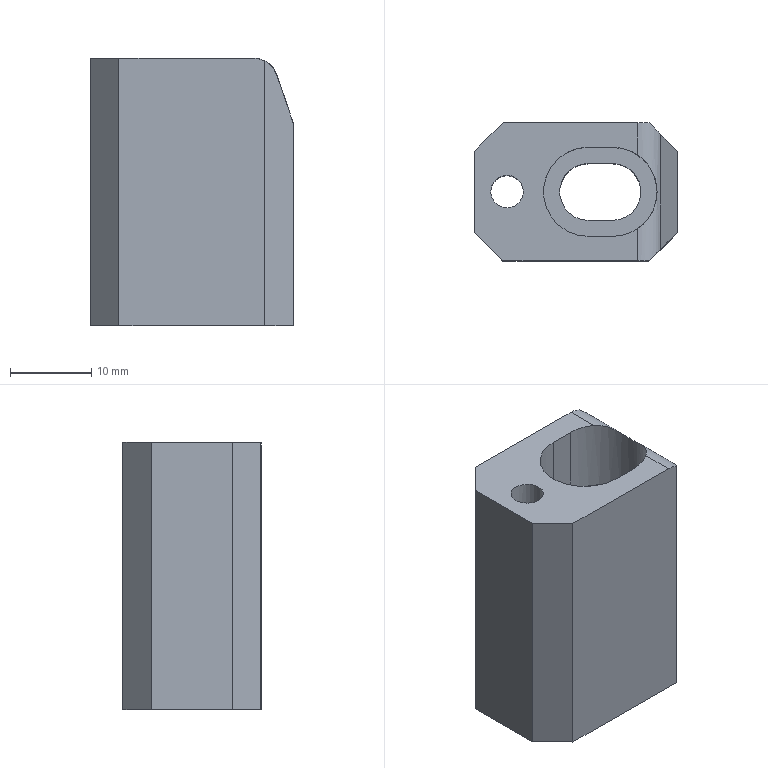Part | NX | features solid 2 | 1 solid | 22 faces | box 25.017 x 17.031 x 33 mm | volume 10081 mm3 | plane 16 | cylinder 6 | commonest cylinder face diameters 7 x2 11 x2 4.001 x1 6 x1
STEP:
#1=CARTESIAN_POINT('',(1242.818,304.277,11.5));
#2=VERTEX_POINT('',#1);
#3=CARTESIAN_POINT('',(1259.419,304.248,11.5));
#4=VERTEX_POINT('',#3);
#5=CARTESIAN_POINT('',(1254.318,304.257,11.5));
#6=DIRECTION('',(1.,-0.001746,0.));
#7=VECTOR('',#6,1000.);
#8=LINE('',#5,#7);
#9=EDGE_CURVE('',#2,#4,#8,.T.);
#10=ORIENTED_EDGE('',*,*,#9,.T.);
#11=CARTESIAN_POINT('',(1259.426,308.205,11.5));
#12=VERTEX_POINT('',#11);
#13=CARTESIAN_POINT('',(1259.434,312.748,11.5));
#14=DIRECTION('',(-0.001746,-1.,0.));
#15=VECTOR('',#14,1000.);
#16=LINE('',#13,#15);
#17=EDGE_CURVE('',#12,#4,#16,.T.);
#18=ORIENTED_EDGE('',*,*,#17,.F.);
#19=CARTESIAN_POINT('',(1256.323,307.253,11.5));
#20=VERTEX_POINT('',#19);
#21=CARTESIAN_POINT('',(1256.333,312.753,11.5));
#22=DIRECTION('',(0.,0.,1.));
#23=DIRECTION('',(-0.165,-0.9863,0.));
#24=AXIS2_PLACEMENT_3D('',#21,#22,#23);
#25=CIRCLE('',#24,5.5);
#26=EDGE_CURVE('',#20,#12,#25,.T.);
#27=ORIENTED_EDGE('',*,*,#26,.F.);
#28=CARTESIAN_POINT('',(1253.323,307.258,11.5));
#29=VERTEX_POINT('',#28);
#30=CARTESIAN_POINT('',(1254.323,307.257,11.5));
#31=DIRECTION('',(1.,-0.001746,0.));
#32=VECTOR('',#31,1000.);
#33=LINE('',#30,#32);
#34=EDGE_CURVE('',#29,#20,#33,.T.);
#35=ORIENTED_EDGE('',*,*,#34,.F.);
#36=CARTESIAN_POINT('',(1253.342,318.258,11.5));
#37=VERTEX_POINT('',#36);
#38=CARTESIAN_POINT('',(1253.333,312.758,11.5));
#39=DIRECTION('',(0.,0.,1.));
#40=DIRECTION('',(-0.165,-0.9863,0.));
#41=AXIS2_PLACEMENT_3D('',#38,#39,#40);
#42=CIRCLE('',#41,5.5);
#43=EDGE_CURVE('',#37,#29,#42,.T.);
#44=ORIENTED_EDGE('',*,*,#43,.F.);
#45=CARTESIAN_POINT('',(1256.342,318.253,11.5));
#46=VERTEX_POINT('',#45);
#47=CARTESIAN_POINT('',(1254.342,318.257,11.5));
#48=DIRECTION('',(-1.,0.001746,0.));
#49=VECTOR('',#48,1000.);
#50=LINE('',#47,#49);
#51=EDGE_CURVE('',#46,#37,#50,.T.);
#52=ORIENTED_EDGE('',*,*,#51,.F.);
#53=CARTESIAN_POINT('',(1259.442,317.29,11.5));
#54=VERTEX_POINT('',#53);
#55=CARTESIAN_POINT('',(1256.333,312.753,11.5));
#56=DIRECTION('',(0.,0.,1.));
#57=DIRECTION('',(-0.165,-0.9863,0.));
#58=AXIS2_PLACEMENT_3D('',#55,#56,#57);
#59=CIRCLE('',#58,5.5);
#60=EDGE_CURVE('',#54,#46,#59,.T.);
#61=ORIENTED_EDGE('',*,*,#60,.F.);
#62=CARTESIAN_POINT('',(1259.449,321.248,11.5));
#63=VERTEX_POINT('',#62);
#64=CARTESIAN_POINT('',(1259.434,312.748,11.5));
#65=DIRECTION('',(-0.001746,-1.,0.));
#66=VECTOR('',#65,1000.);
#67=LINE('',#64,#66);
#68=EDGE_CURVE('',#63,#54,#67,.T.);
#69=ORIENTED_EDGE('',*,*,#68,.F.);
#70=CARTESIAN_POINT('',(1242.848,321.277,11.5));
#71=VERTEX_POINT('',#70);
#72=CARTESIAN_POINT('',(1254.348,321.257,11.5));
#73=DIRECTION('',(-1.,0.001746,0.));
#74=VECTOR('',#73,1000.);
#75=LINE('',#72,#74);
#76=EDGE_CURVE('',#63,#71,#75,.T.);
#77=ORIENTED_EDGE('',*,*,#76,.T.);
#78=CARTESIAN_POINT('',(1239.342,317.783,11.5));
#79=VERTEX_POINT('',#78);
#80=CARTESIAN_POINT('',(1243.849,322.275,11.5));
#81=DIRECTION('',(0.7083,0.7059,0.));
#82=VECTOR('',#81,1000.);
#83=LINE('',#80,#82);
#84=EDGE_CURVE('',#79,#71,#83,.T.);
#85=ORIENTED_EDGE('',*,*,#84,.F.);
#86=CARTESIAN_POINT('',(1239.324,307.783,11.5));
#87=VERTEX_POINT('',#86);
#88=CARTESIAN_POINT('',(1239.333,312.783,11.5));
#89=DIRECTION('',(-0.001746,-1.,0.));
#90=VECTOR('',#89,1000.);
#91=LINE('',#88,#90);
#92=EDGE_CURVE('',#79,#87,#91,.T.);
#93=ORIENTED_EDGE('',*,*,#92,.T.);
#94=CARTESIAN_POINT('',(1243.816,303.275,11.5));
#95=DIRECTION('',(-0.7059,0.7083,0.));
#96=VECTOR('',#95,1000.);
#97=LINE('',#94,#96);
#98=EDGE_CURVE('',#2,#87,#97,.T.);
#99=ORIENTED_EDGE('',*,*,#98,.F.);
#100=EDGE_LOOP('',(#10,#18,#27,#35,#44,#52,#61,#69,#77,#85,#93,#99));
#101=FACE_BOUND('',#100,.T.);
#102=CARTESIAN_POINT('',(1242.873,314.723,11.5));
#103=VERTEX_POINT('',#102);
#104=CARTESIAN_POINT('',(1243.333,312.776,11.5));
#105=DIRECTION('',(0.,0.,1.));
#106=DIRECTION('',(-0.23,0.9732,0.));
#107=AXIS2_PLACEMENT_3D('',#104,#105,#106);
#108=CIRCLE('',#107,2.001);
#109=EDGE_CURVE('',#103,#103,#108,.T.);
#110=ORIENTED_EDGE('',*,*,#109,.F.);
#111=EDGE_LOOP('',(#110));
#112=FACE_BOUND('',#111,.T.);
#113=CARTESIAN_POINT('',(1254.333,312.757,11.5));
#114=DIRECTION('',(0.,0.,1.));
#115=DIRECTION('',(0.1754,0.9845,0.));
#116=AXIS2_PLACEMENT_3D('',#113,#114,#115);
#117=PLANE('',#116);
#118=ADVANCED_FACE('',(#101,#112),#117,.T.);
#119=CARTESIAN_POINT('',(1243.8,314.721,-21.5));
#120=VERTEX_POINT('',#119);
#121=CARTESIAN_POINT('',(1243.333,312.776,-21.5));
#122=DIRECTION('',(0.,0.,1.));
#123=DIRECTION('',(0.2334,0.9724,0.));
#124=AXIS2_PLACEMENT_3D('',#121,#122,#123);
#125=CIRCLE('',#124,2.001);
#126=EDGE_CURVE('',#120,#120,#125,.T.);
#127=ORIENTED_EDGE('',*,*,#126,.T.);
#128=EDGE_LOOP('',(#127));
#129=FACE_BOUND('',#128,.T.);
#130=CARTESIAN_POINT('',(1260.818,304.245,-21.5));
#131=VERTEX_POINT('',#130);
#132=CARTESIAN_POINT('',(1242.818,304.277,-21.5));
#133=VERTEX_POINT('',#132);
#134=CARTESIAN_POINT('',(1254.318,304.257,-21.5));
#135=DIRECTION('',(-1.,0.001746,0.));
#136=VECTOR('',#135,1000.);
#137=LINE('',#134,#136);
#138=EDGE_CURVE('',#131,#133,#137,.T.);
#139=ORIENTED_EDGE('',*,*,#138,.T.);
#140=CARTESIAN_POINT('',(1239.324,307.783,-21.5));
#141=VERTEX_POINT('',#140);
#142=CARTESIAN_POINT('',(1243.317,303.776,-21.5));
#143=DIRECTION('',(0.7059,-0.7083,0.));
#144=VECTOR('',#143,1000.);
#145=LINE('',#142,#144);
#146=EDGE_CURVE('',#141,#133,#145,.T.);
#147=ORIENTED_EDGE('',*,*,#146,.F.);
#148=CARTESIAN_POINT('',(1239.342,317.783,-21.5));
#149=VERTEX_POINT('',#148);
#150=CARTESIAN_POINT('',(1239.333,312.783,-21.5));
#151=DIRECTION('',(0.001746,1.,0.));
#152=VECTOR('',#151,1000.);
#153=LINE('',#150,#152);
#154=EDGE_CURVE('',#141,#149,#153,.T.);
#155=ORIENTED_EDGE('',*,*,#154,.T.);
#156=CARTESIAN_POINT('',(1242.848,321.277,-21.5));
#157=VERTEX_POINT('',#156);
#158=CARTESIAN_POINT('',(1243.349,321.776,-21.5));
#159=DIRECTION('',(-0.7083,-0.7059,0.));
#160=VECTOR('',#159,1000.);
#161=LINE('',#158,#160);
#162=EDGE_CURVE('',#157,#149,#161,.T.);
#163=ORIENTED_EDGE('',*,*,#162,.F.);
#164=CARTESIAN_POINT('',(1260.848,321.245,-21.5));
#165=VERTEX_POINT('',#164);
#166=CARTESIAN_POINT('',(1254.348,321.257,-21.5));
#167=DIRECTION('',(1.,-0.001746,0.));
#168=VECTOR('',#167,1000.);
#169=LINE('',#166,#168);
#170=EDGE_CURVE('',#157,#165,#169,.T.);
#171=ORIENTED_EDGE('',*,*,#170,.T.);
#172=CARTESIAN_POINT('',(1264.342,317.739,-21.5));
#173=VERTEX_POINT('',#172);
#174=CARTESIAN_POINT('',(1261.846,320.243,-21.5));
#175=DIRECTION('',(-0.7059,0.7083,0.));
#176=VECTOR('',#175,1000.);
#177=LINE('',#174,#176);
#178=EDGE_CURVE('',#173,#165,#177,.T.);
#179=ORIENTED_EDGE('',*,*,#178,.F.);
#180=CARTESIAN_POINT('',(1264.324,307.739,-21.5));
#181=VERTEX_POINT('',#180);
#182=CARTESIAN_POINT('',(1264.333,312.739,-21.5));
#183=DIRECTION('',(-0.001746,-1.,0.));
#184=VECTOR('',#183,1000.);
#185=LINE('',#182,#184);
#186=EDGE_CURVE('',#173,#181,#185,.T.);
#187=ORIENTED_EDGE('',*,*,#186,.T.);
#188=CARTESIAN_POINT('',(1261.82,305.243,-21.5));
#189=DIRECTION('',(0.7083,0.7059,0.));
#190=VECTOR('',#189,1000.);
#191=LINE('',#188,#190);
#192=EDGE_CURVE('',#131,#181,#191,.T.);
#193=ORIENTED_EDGE('',*,*,#192,.F.);
#194=EDGE_LOOP('',(#139,#147,#155,#163,#171,#179,#187,#193));
#195=FACE_BOUND('',#194,.T.);
#196=CARTESIAN_POINT('',(1256.339,316.253,-21.5));
#197=VERTEX_POINT('',#196);
#198=CARTESIAN_POINT('',(1256.327,309.253,-21.5));
#199=VERTEX_POINT('',#198);
#200=CARTESIAN_POINT('',(1256.333,312.753,-21.5));
#201=DIRECTION('',(0.,0.,-1.));
#202=DIRECTION('',(0.2334,0.9724,0.));
#203=AXIS2_PLACEMENT_3D('',#200,#201,#202);
#204=CIRCLE('',#203,3.5);
#205=EDGE_CURVE('',#197,#199,#204,.T.);
#206=ORIENTED_EDGE('',*,*,#205,.F.);
#207=CARTESIAN_POINT('',(1253.339,316.258,-21.5));
#208=VERTEX_POINT('',#207);
#209=CARTESIAN_POINT('',(1254.339,316.257,-21.5));
#210=DIRECTION('',(1.,-0.001746,0.));
#211=VECTOR('',#210,1000.);
#212=LINE('',#209,#211);
#213=EDGE_CURVE('',#208,#197,#212,.T.);
#214=ORIENTED_EDGE('',*,*,#213,.F.);
#215=CARTESIAN_POINT('',(1253.327,309.258,-21.5));
#216=VERTEX_POINT('',#215);
#217=CARTESIAN_POINT('',(1253.333,312.758,-21.5));
#218=DIRECTION('',(0.,0.,-1.));
#219=DIRECTION('',(0.2334,0.9724,0.));
#220=AXIS2_PLACEMENT_3D('',#217,#218,#219);
#221=CIRCLE('',#220,3.5);
#222=EDGE_CURVE('',#216,#208,#221,.T.);
#223=ORIENTED_EDGE('',*,*,#222,.F.);
#224=CARTESIAN_POINT('',(1254.327,309.257,-21.5));
#225=DIRECTION('',(-1.,0.001746,0.));
#226=VECTOR('',#225,1000.);
#227=LINE('',#224,#226);
#228=EDGE_CURVE('',#199,#216,#227,.T.);
#229=ORIENTED_EDGE('',*,*,#228,.F.);
#230=EDGE_LOOP('',(#206,#214,#223,#229));
#231=FACE_BOUND('',#230,.T.);
#232=CARTESIAN_POINT('',(1254.333,312.757,-21.5));
#233=DIRECTION('',(0.,0.,-1.));
#234=DIRECTION('',(-0.1754,-0.9845,0.));
#235=AXIS2_PLACEMENT_3D('',#232,#233,#234);
#236=PLANE('',#235);
#237=ADVANCED_FACE('',(#129,#195,#231),#236,.T.);
#238=ORIENTED_EDGE('',*,*,#186,.F.);
#239=CARTESIAN_POINT('',(1264.342,317.739,3.5));
#240=VERTEX_POINT('',#239);
#241=CARTESIAN_POINT('',(1264.342,317.739,-13.5));
#242=DIRECTION('',(0.,0.,-1.));
#243=VECTOR('',#242,1000.);
#244=LINE('',#241,#243);
#245=EDGE_CURVE('',#240,#173,#244,.T.);
#246=ORIENTED_EDGE('',*,*,#245,.F.);
#247=CARTESIAN_POINT('',(1264.324,307.739,3.5));
#248=VERTEX_POINT('',#247);
#249=CARTESIAN_POINT('',(1264.333,312.739,3.5));
#250=DIRECTION('',(0.001746,1.,0.));
#251=VECTOR('',#250,1000.);
#252=LINE('',#249,#251);
#253=EDGE_CURVE('',#248,#240,#252,.T.);
#254=ORIENTED_EDGE('',*,*,#253,.F.);
#255=CARTESIAN_POINT('',(1264.324,307.739,-13.5));
#256=DIRECTION('',(0.,0.,1.));
#257=VECTOR('',#256,1000.);
#258=LINE('',#255,#257);
#259=EDGE_CURVE('',#181,#248,#258,.T.);
#260=ORIENTED_EDGE('',*,*,#259,.F.);
#261=EDGE_LOOP('',(#238,#246,#254,#260));
#262=FACE_BOUND('',#261,.T.);
#263=CARTESIAN_POINT('',(1264.333,312.739,-13.5));
#264=DIRECTION('',(1.,-0.001746,0.));
#265=DIRECTION('',(0.001746,1.,0.));
#266=AXIS2_PLACEMENT_3D('',#263,#264,#265);
#267=PLANE('',#266);
#268=ADVANCED_FACE('',(#262),#267,.T.);
#269=ORIENTED_EDGE('',*,*,#170,.F.);
#270=CARTESIAN_POINT('',(1242.848,321.277,-13.5));
#271=DIRECTION('',(0.,0.,-1.));
#272=VECTOR('',#271,1000.);
#273=LINE('',#270,#272);
#274=EDGE_CURVE('',#71,#157,#273,.T.);
#275=ORIENTED_EDGE('',*,*,#274,.F.);
#276=ORIENTED_EDGE('',*,*,#76,.F.);
#277=CARTESIAN_POINT('',(1260.848,321.245,11.154));
#278=VERTEX_POINT('',#277);
#279=CARTESIAN_POINT('',(1259.449,321.248,8.5));
#280=DIRECTION('',(-0.001746,-1.,0.));
#281=DIRECTION('',(-1.,0.001746,0.));
#282=AXIS2_PLACEMENT_3D('',#279,#280,#281);
#283=CIRCLE('',#282,3.);
#284=EDGE_CURVE('',#278,#63,#283,.T.);
#285=ORIENTED_EDGE('',*,*,#284,.F.);
#286=CARTESIAN_POINT('',(1260.848,321.245,-13.5));
#287=DIRECTION('',(0.,0.,1.));
#288=VECTOR('',#287,1000.);
#289=LINE('',#286,#288);
#290=EDGE_CURVE('',#165,#278,#289,.T.);
#291=ORIENTED_EDGE('',*,*,#290,.F.);
#292=EDGE_LOOP('',(#269,#275,#276,#285,#291));
#293=FACE_BOUND('',#292,.T.);
#294=CARTESIAN_POINT('',(1254.348,321.257,-13.5));
#295=DIRECTION('',(0.001746,1.,0.));
#296=DIRECTION('',(-1.,0.001746,0.));
#297=AXIS2_PLACEMENT_3D('',#294,#295,#296);
#298=PLANE('',#297);
#299=ADVANCED_FACE('',(#293),#298,.T.);
#300=ORIENTED_EDGE('',*,*,#92,.F.);
#301=CARTESIAN_POINT('',(1239.342,317.783,-13.5));
#302=DIRECTION('',(0.,0.,1.));
#303=VECTOR('',#302,1000.);
#304=LINE('',#301,#303);
#305=EDGE_CURVE('',#149,#79,#304,.T.);
#306=ORIENTED_EDGE('',*,*,#305,.F.);
#307=ORIENTED_EDGE('',*,*,#154,.F.);
#308=CARTESIAN_POINT('',(1239.324,307.783,-13.5));
#309=DIRECTION('',(0.,0.,-1.));
#310=VECTOR('',#309,1000.);
#311=LINE('',#308,#310);
#312=EDGE_CURVE('',#87,#141,#311,.T.);
#313=ORIENTED_EDGE('',*,*,#312,.F.);
#314=EDGE_LOOP('',(#300,#306,#307,#313));
#315=FACE_BOUND('',#314,.T.);
#316=CARTESIAN_POINT('',(1239.333,312.783,-13.5));
#317=DIRECTION('',(-1.,0.001746,0.));
#318=DIRECTION('',(-0.001746,-1.,0.));
#319=AXIS2_PLACEMENT_3D('',#316,#317,#318);
#320=PLANE('',#319);
#321=ADVANCED_FACE('',(#315),#320,.T.);
#322=CARTESIAN_POINT('',(1260.818,304.245,11.154));
#323=VERTEX_POINT('',#322);
#324=CARTESIAN_POINT('',(1259.419,304.248,8.5));
#325=DIRECTION('',(0.001746,1.,0.));
#326=DIRECTION('',(1.,-0.001746,0.));
#327=AXIS2_PLACEMENT_3D('',#324,#325,#326);
#328=CIRCLE('',#327,3.);
#329=EDGE_CURVE('',#4,#323,#328,.T.);
#330=ORIENTED_EDGE('',*,*,#329,.F.);
#331=ORIENTED_EDGE('',*,*,#9,.F.);
#332=CARTESIAN_POINT('',(1242.818,304.277,-13.5));
#333=DIRECTION('',(0.,0.,1.));
#334=VECTOR('',#333,1000.);
#335=LINE('',#332,#334);
#336=EDGE_CURVE('',#133,#2,#335,.T.);
#337=ORIENTED_EDGE('',*,*,#336,.F.);
#338=ORIENTED_EDGE('',*,*,#138,.F.);
#339=CARTESIAN_POINT('',(1260.818,304.245,-13.5));
#340=DIRECTION('',(0.,0.,-1.));
#341=VECTOR('',#340,1000.);
#342=LINE('',#339,#341);
#343=EDGE_CURVE('',#323,#131,#342,.T.);
#344=ORIENTED_EDGE('',*,*,#343,.F.);
#345=EDGE_LOOP('',(#330,#331,#337,#338,#344));
#346=FACE_BOUND('',#345,.T.);
#347=CARTESIAN_POINT('',(1254.318,304.257,-13.5));
#348=DIRECTION('',(-0.001746,-1.,0.));
#349=DIRECTION('',(1.,-0.001746,0.));
#350=AXIS2_PLACEMENT_3D('',#347,#348,#349);
#351=PLANE('',#350);
#352=ADVANCED_FACE('',(#346),#351,.T.);
#353=CARTESIAN_POINT('',(1253.327,309.258,2.5));
#354=VERTEX_POINT('',#353);
#355=CARTESIAN_POINT('',(1253.339,316.258,2.5));
#356=VERTEX_POINT('',#355);
#357=CARTESIAN_POINT('',(1253.333,312.758,2.5));
#358=DIRECTION('',(0.,0.,-1.));
#359=DIRECTION('',(0.165,0.9863,0.));
#360=AXIS2_PLACEMENT_3D('',#357,#358,#359);
#361=CIRCLE('',#360,3.5);
#362=EDGE_CURVE('',#354,#356,#361,.T.);
#363=ORIENTED_EDGE('',*,*,#362,.T.);
#364=CARTESIAN_POINT('',(1256.339,316.253,2.5));
#365=VERTEX_POINT('',#364);
#366=CARTESIAN_POINT('',(1253.437,316.258,2.5));
#367=DIRECTION('',(-1.,0.001746,0.));
#368=VECTOR('',#367,1000.);
#369=LINE('',#366,#368);
#370=EDGE_CURVE('',#365,#356,#369,.T.);
#371=ORIENTED_EDGE('',*,*,#370,.F.);
#372=CARTESIAN_POINT('',(1256.327,309.253,2.5));
#373=VERTEX_POINT('',#372);
#374=CARTESIAN_POINT('',(1256.333,312.753,2.5));
#375=DIRECTION('',(0.,0.,1.));
#376=DIRECTION('',(0.165,0.9863,0.));
#377=AXIS2_PLACEMENT_3D('',#374,#375,#376);
#378=CIRCLE('',#377,3.5);
#379=EDGE_CURVE('',#373,#365,#378,.T.);
#380=ORIENTED_EDGE('',*,*,#379,.F.);
#381=CARTESIAN_POINT('',(1253.425,309.258,2.5));
#382=DIRECTION('',(1.,-0.001746,0.));
#383=VECTOR('',#382,1000.);
#384=LINE('',#381,#383);
#385=EDGE_CURVE('',#354,#373,#384,.T.);
#386=ORIENTED_EDGE('',*,*,#385,.F.);
#387=EDGE_LOOP('',(#363,#371,#380,#386));
#388=FACE_BOUND('',#387,.T.);
#389=CARTESIAN_POINT('',(1256.323,307.253,2.5));
#390=VERTEX_POINT('',#389);
#391=CARTESIAN_POINT('',(1256.342,318.253,2.5));
#392=VERTEX_POINT('',#391);
#393=CARTESIAN_POINT('',(1256.333,312.753,2.5));
#394=DIRECTION('',(0.,0.,1.));
#395=DIRECTION('',(0.165,0.9863,0.));
#396=AXIS2_PLACEMENT_3D('',#393,#394,#395);
#397=CIRCLE('',#396,5.5);
#398=EDGE_CURVE('',#390,#392,#397,.T.);
#399=ORIENTED_EDGE('',*,*,#398,.T.);
#400=CARTESIAN_POINT('',(1253.342,318.258,2.5));
#401=VERTEX_POINT('',#400);
#402=CARTESIAN_POINT('',(1252.342,318.26,2.5));
#403=DIRECTION('',(1.,-0.001746,0.));
#404=VECTOR('',#403,1000.);
#405=LINE('',#402,#404);
#406=EDGE_CURVE('',#401,#392,#405,.T.);
#407=ORIENTED_EDGE('',*,*,#406,.F.);
#408=CARTESIAN_POINT('',(1253.323,307.258,2.5));
#409=VERTEX_POINT('',#408);
#410=CARTESIAN_POINT('',(1253.333,312.758,2.5));
#411=DIRECTION('',(0.,0.,-1.));
#412=DIRECTION('',(0.165,0.9863,0.));
#413=AXIS2_PLACEMENT_3D('',#410,#411,#412);
#414=CIRCLE('',#413,5.5);
#415=EDGE_CURVE('',#409,#401,#414,.T.);
#416=ORIENTED_EDGE('',*,*,#415,.F.);
#417=CARTESIAN_POINT('',(1252.323,307.26,2.5));
#418=DIRECTION('',(-1.,0.001746,0.));
#419=VECTOR('',#418,1000.);
#420=LINE('',#417,#419);
#421=EDGE_CURVE('',#390,#409,#420,.T.);
#422=ORIENTED_EDGE('',*,*,#421,.F.);
#423=EDGE_LOOP('',(#399,#407,#416,#422));
#424=FACE_BOUND('',#423,.T.);
#425=CARTESIAN_POINT('',(1252.333,312.76,2.5));
#426=DIRECTION('',(0.,0.,-1.));
#427=DIRECTION('',(-0.165,-0.9863,0.));
#428=AXIS2_PLACEMENT_3D('',#425,#426,#427);
#429=PLANE('',#428);
#430=ADVANCED_FACE('',(#388,#424),#429,.F.);
#431=ORIENTED_EDGE('',*,*,#222,.T.);
#432=CARTESIAN_POINT('',(1253.339,316.258,-10.5));
#433=DIRECTION('',(0.,0.,-1.));
#434=VECTOR('',#433,1000.);
#435=LINE('',#432,#434);
#436=EDGE_CURVE('',#356,#208,#435,.T.);
#437=ORIENTED_EDGE('',*,*,#436,.F.);
#438=ORIENTED_EDGE('',*,*,#362,.F.);
#439=CARTESIAN_POINT('',(1253.327,309.258,-10.5));
#440=DIRECTION('',(0.,0.,1.));
#441=VECTOR('',#440,1000.);
#442=LINE('',#439,#441);
#443=EDGE_CURVE('',#216,#354,#442,.T.);
#444=ORIENTED_EDGE('',*,*,#443,.F.);
#445=EDGE_LOOP('',(#431,#437,#438,#444));
#446=FACE_BOUND('',#445,.T.);
#447=CARTESIAN_POINT('',(1253.333,312.758,6.5));
#448=DIRECTION('',(0.,0.,-1.));
#449=DIRECTION('',(0.165,0.9863,0.));
#450=AXIS2_PLACEMENT_3D('',#447,#448,#449);
#451=CYLINDRICAL_SURFACE('',#450,3.5);
#452=ADVANCED_FACE('',(#446),#451,.F.);
#453=ORIENTED_EDGE('',*,*,#415,.T.);
#454=CARTESIAN_POINT('',(1253.342,318.258,7.));
#455=DIRECTION('',(0.,0.,-1.));
#456=VECTOR('',#455,1000.);
#457=LINE('',#454,#456);
#458=EDGE_CURVE('',#37,#401,#457,.T.);
#459=ORIENTED_EDGE('',*,*,#458,.F.);
#460=ORIENTED_EDGE('',*,*,#43,.T.);
#461=CARTESIAN_POINT('',(1253.323,307.258,7.));
#462=DIRECTION('',(0.,0.,1.));
#463=VECTOR('',#462,1000.);
#464=LINE('',#461,#463);
#465=EDGE_CURVE('',#409,#29,#464,.T.);
#466=ORIENTED_EDGE('',*,*,#465,.F.);
#467=EDGE_LOOP('',(#453,#459,#460,#466));
#468=FACE_BOUND('',#467,.T.);
#469=CARTESIAN_POINT('',(1253.333,312.758,16.5));
#470=DIRECTION('',(0.,0.,-1.));
#471=DIRECTION('',(0.165,0.9863,0.));
#472=AXIS2_PLACEMENT_3D('',#469,#470,#471);
#473=CYLINDRICAL_SURFACE('',#472,5.5);
#474=ADVANCED_FACE('',(#468),#473,.F.);
#475=ORIENTED_EDGE('',*,*,#379,.T.);
#476=CARTESIAN_POINT('',(1256.339,316.253,-10.5));
#477=DIRECTION('',(0.,0.,1.));
#478=VECTOR('',#477,1000.);
#479=LINE('',#476,#478);
#480=EDGE_CURVE('',#197,#365,#479,.T.);
#481=ORIENTED_EDGE('',*,*,#480,.F.);
#482=ORIENTED_EDGE('',*,*,#205,.T.);
#483=CARTESIAN_POINT('',(1256.327,309.253,-10.5));
#484=DIRECTION('',(0.,0.,-1.));
#485=VECTOR('',#484,1000.);
#486=LINE('',#483,#485);
#487=EDGE_CURVE('',#373,#199,#486,.T.);
#488=ORIENTED_EDGE('',*,*,#487,.F.);
#489=EDGE_LOOP('',(#475,#481,#482,#488));
#490=FACE_BOUND('',#489,.T.);
#491=CARTESIAN_POINT('',(1256.333,312.753,6.5));
#492=DIRECTION('',(0.,0.,-1.));
#493=DIRECTION('',(0.165,0.9863,0.));
#494=AXIS2_PLACEMENT_3D('',#491,#492,#493);
#495=CYLINDRICAL_SURFACE('',#494,3.5);
#496=ADVANCED_FACE('',(#490),#495,.F.);
#497=ORIENTED_EDGE('',*,*,#26,.T.);
#498=CARTESIAN_POINT('',(1259.442,317.29,11.5));
#499=CARTESIAN_POINT('',(1260.209,316.764,11.5));
#500=CARTESIAN_POINT('',(1261.383,315.42,10.952));
#501=CARTESIAN_POINT('',(1262.06,312.742,9.976));
#502=CARTESIAN_POINT('',(1261.374,310.069,10.952));
#503=CARTESIAN_POINT('',(1260.195,308.728,11.5));
#504=CARTESIAN_POINT('',(1259.426,308.205,11.5));
#505=B_SPLINE_CURVE_WITH_KNOTS('',3,(#498,#499,#500,#501,#502,#503,#504),.UNSPECIFIED.,.F.,.F.,(4,1,1,1,4),(0.,0.002735,0.00547,0.008205,0.01094),.UNSPECIFIED.);
#506=EDGE_CURVE('',#54,#12,#505,.T.);
#507=ORIENTED_EDGE('',*,*,#506,.F.);
#508=ORIENTED_EDGE('',*,*,#60,.T.);
#509=CARTESIAN_POINT('',(1256.342,318.253,7.));
#510=DIRECTION('',(0.,0.,1.));
#511=VECTOR('',#510,1000.);
#512=LINE('',#509,#511);
#513=EDGE_CURVE('',#392,#46,#512,.T.);
#514=ORIENTED_EDGE('',*,*,#513,.F.);
#515=ORIENTED_EDGE('',*,*,#398,.F.);
#516=CARTESIAN_POINT('',(1256.323,307.253,7.));
#517=DIRECTION('',(0.,0.,-1.));
#518=VECTOR('',#517,1000.);
#519=LINE('',#516,#518);
#520=EDGE_CURVE('',#20,#390,#519,.T.);
#521=ORIENTED_EDGE('',*,*,#520,.F.);
#522=EDGE_LOOP('',(#497,#507,#508,#514,#515,#521));
#523=FACE_BOUND('',#522,.T.);
#524=CARTESIAN_POINT('',(1256.333,312.753,16.5));
#525=DIRECTION('',(0.,0.,-1.));
#526=DIRECTION('',(0.165,0.9863,0.));
#527=AXIS2_PLACEMENT_3D('',#524,#525,#526);
#528=CYLINDRICAL_SURFACE('',#527,5.5);
#529=ADVANCED_FACE('',(#523),#528,.F.);
#530=ORIENTED_EDGE('',*,*,#253,.T.);
#531=CARTESIAN_POINT('',(1262.282,319.805,9.478));
#532=VERTEX_POINT('',#531);
#533=CARTESIAN_POINT('',(1268.495,313.571,-8.559));
#534=DIRECTION('',(0.3095,-0.3106,-0.8987));
#535=VECTOR('',#534,1000.);
#536=LINE('',#533,#535);
#537=EDGE_CURVE('',#532,#240,#536,.T.);
#538=ORIENTED_EDGE('',*,*,#537,.F.);
#539=CARTESIAN_POINT('',(1262.258,305.68,9.478));
#540=VERTEX_POINT('',#539);
#541=CARTESIAN_POINT('',(1262.27,312.743,9.478));
#542=DIRECTION('',(0.001746,1.,0.));
#543=VECTOR('',#542,1000.);
#544=LINE('',#541,#543);
#545=EDGE_CURVE('',#540,#532,#544,.T.);
#546=ORIENTED_EDGE('',*,*,#545,.F.);
#547=CARTESIAN_POINT('',(1269.07,312.468,-10.231));
#548=DIRECTION('',(-0.3106,-0.3095,0.8987));
#549=VECTOR('',#548,1000.);
#550=LINE('',#547,#549);
#551=EDGE_CURVE('',#248,#540,#550,.T.);
#552=ORIENTED_EDGE('',*,*,#551,.F.);
#553=EDGE_LOOP('',(#530,#538,#546,#552));
#554=FACE_BOUND('',#553,.T.);
#555=CARTESIAN_POINT('',(1264.333,312.739,3.5));
#556=DIRECTION('',(-0.9453,0.00165,-0.3262));
#557=DIRECTION('',(-0.001746,-1.,0.));
#558=AXIS2_PLACEMENT_3D('',#555,#556,#557);
#559=PLANE('',#558);
#560=ADVANCED_FACE('',(#554),#559,.F.);
#561=ORIENTED_EDGE('',*,*,#545,.T.);
#562=CARTESIAN_POINT('',(1259.451,322.646,8.5));
#563=DIRECTION('',(0.7083,0.7059,0.));
#564=DIRECTION('',(-0.7059,0.7083,0.));
#565=AXIS2_PLACEMENT_3D('',#562,#563,#564);
#566=ELLIPSE('',#565,4.243,3.);
#567=EDGE_CURVE('',#278,#532,#566,.T.);
#568=ORIENTED_EDGE('',*,*,#567,.F.);
#569=ORIENTED_EDGE('',*,*,#284,.T.);
#570=ORIENTED_EDGE('',*,*,#68,.T.);
#571=ORIENTED_EDGE('',*,*,#506,.T.);
#572=ORIENTED_EDGE('',*,*,#17,.T.);
#573=ORIENTED_EDGE('',*,*,#329,.T.);
#574=CARTESIAN_POINT('',(1259.417,302.849,8.5));
#575=DIRECTION('',(0.7059,-0.7083,0.));
#576=DIRECTION('',(0.7083,0.7059,0.));
#577=AXIS2_PLACEMENT_3D('',#574,#575,#576);
#578=ELLIPSE('',#577,4.243,3.);
#579=EDGE_CURVE('',#540,#323,#578,.T.);
#580=ORIENTED_EDGE('',*,*,#579,.F.);
#581=EDGE_LOOP('',(#561,#568,#569,#570,#571,#572,#573,#580));
#582=FACE_BOUND('',#581,.T.);
#583=CARTESIAN_POINT('',(1259.434,312.748,8.5));
#584=DIRECTION('',(0.001746,1.,0.));
#585=DIRECTION('',(-1.,0.001746,0.));
#586=AXIS2_PLACEMENT_3D('',#583,#584,#585);
#587=CYLINDRICAL_SURFACE('',#586,3.);
#588=ADVANCED_FACE('',(#582),#587,.T.);
#589=ORIENTED_EDGE('',*,*,#51,.T.);
#590=ORIENTED_EDGE('',*,*,#458,.T.);
#591=ORIENTED_EDGE('',*,*,#406,.T.);
#592=ORIENTED_EDGE('',*,*,#513,.T.);
#593=EDGE_LOOP('',(#589,#590,#591,#592));
#594=FACE_BOUND('',#593,.T.);
#595=CARTESIAN_POINT('',(1253.378,318.258,16.5));
#596=DIRECTION('',(0.001746,1.,0.));
#597=DIRECTION('',(0.,0.,1.));
#598=AXIS2_PLACEMENT_3D('',#595,#596,#597);
#599=PLANE('',#598);
#600=ADVANCED_FACE('',(#594),#599,.F.);
#601=ORIENTED_EDGE('',*,*,#370,.T.);
#602=ORIENTED_EDGE('',*,*,#436,.T.);
#603=ORIENTED_EDGE('',*,*,#213,.T.);
#604=ORIENTED_EDGE('',*,*,#480,.T.);
#605=EDGE_LOOP('',(#601,#602,#603,#604));
#606=FACE_BOUND('',#605,.T.);
#607=CARTESIAN_POINT('',(1253.437,316.258,6.5));
#608=DIRECTION('',(0.001746,1.,0.));
#609=DIRECTION('',(0.,0.,1.));
#610=AXIS2_PLACEMENT_3D('',#607,#608,#609);
#611=PLANE('',#610);
#612=ADVANCED_FACE('',(#606),#611,.F.);
#613=ORIENTED_EDGE('',*,*,#228,.T.);
#614=ORIENTED_EDGE('',*,*,#443,.T.);
#615=ORIENTED_EDGE('',*,*,#385,.T.);
#616=ORIENTED_EDGE('',*,*,#487,.T.);
#617=EDGE_LOOP('',(#613,#614,#615,#616));
#618=FACE_BOUND('',#617,.T.);
#619=CARTESIAN_POINT('',(1253.425,309.258,6.5));
#620=DIRECTION('',(-0.001746,-1.,0.));
#621=DIRECTION('',(0.,0.,-1.));
#622=AXIS2_PLACEMENT_3D('',#619,#620,#621);
#623=PLANE('',#622);
#624=ADVANCED_FACE('',(#618),#623,.F.);
#625=ORIENTED_EDGE('',*,*,#421,.T.);
#626=ORIENTED_EDGE('',*,*,#465,.T.);
#627=ORIENTED_EDGE('',*,*,#34,.T.);
#628=ORIENTED_EDGE('',*,*,#520,.T.);
#629=EDGE_LOOP('',(#625,#626,#627,#628));
#630=FACE_BOUND('',#629,.T.);
#631=CARTESIAN_POINT('',(1253.359,307.258,16.5));
#632=DIRECTION('',(-0.001746,-1.,0.));
#633=DIRECTION('',(0.,0.,-1.));
#634=AXIS2_PLACEMENT_3D('',#631,#632,#633);
#635=PLANE('',#634);
#636=ADVANCED_FACE('',(#630),#635,.F.);
#637=ORIENTED_EDGE('',*,*,#146,.T.);
#638=ORIENTED_EDGE('',*,*,#336,.T.);
#639=ORIENTED_EDGE('',*,*,#98,.T.);
#640=ORIENTED_EDGE('',*,*,#312,.T.);
#641=EDGE_LOOP('',(#637,#638,#639,#640));
#642=FACE_BOUND('',#641,.T.);
#643=CARTESIAN_POINT('',(1242.319,304.777,-13.5));
#644=DIRECTION('',(0.7083,0.7059,0.));
#645=DIRECTION('',(0.,0.,-1.));
#646=AXIS2_PLACEMENT_3D('',#643,#644,#645);
#647=PLANE('',#646);
#648=ADVANCED_FACE('',(#642),#647,.F.);
#649=ORIENTED_EDGE('',*,*,#162,.T.);
#650=ORIENTED_EDGE('',*,*,#305,.T.);
#651=ORIENTED_EDGE('',*,*,#84,.T.);
#652=ORIENTED_EDGE('',*,*,#274,.T.);
#653=EDGE_LOOP('',(#649,#650,#651,#652));
#654=FACE_BOUND('',#653,.T.);
#655=CARTESIAN_POINT('',(1239.342,317.783,-13.5));
#656=DIRECTION('',(0.7059,-0.7083,0.));
#657=DIRECTION('',(0.,0.,-1.));
#658=AXIS2_PLACEMENT_3D('',#655,#656,#657);
#659=PLANE('',#658);
#660=ADVANCED_FACE('',(#654),#659,.F.);
#661=ORIENTED_EDGE('',*,*,#178,.T.);
#662=ORIENTED_EDGE('',*,*,#290,.T.);
#663=ORIENTED_EDGE('',*,*,#567,.T.);
#664=ORIENTED_EDGE('',*,*,#537,.T.);
#665=ORIENTED_EDGE('',*,*,#245,.T.);
#666=EDGE_LOOP('',(#661,#662,#663,#664,#665));
#667=FACE_BOUND('',#666,.T.);
#668=CARTESIAN_POINT('',(1261.347,320.744,-13.5));
#669=DIRECTION('',(-0.7083,-0.7059,0.));
#670=DIRECTION('',(0.,0.,-1.));
#671=AXIS2_PLACEMENT_3D('',#668,#669,#670);
#672=PLANE('',#671);
#673=ADVANCED_FACE('',(#667),#672,.F.);
#674=ORIENTED_EDGE('',*,*,#192,.T.);
#675=ORIENTED_EDGE('',*,*,#259,.T.);
#676=ORIENTED_EDGE('',*,*,#551,.T.);
#677=ORIENTED_EDGE('',*,*,#579,.T.);
#678=ORIENTED_EDGE('',*,*,#343,.T.);
#679=EDGE_LOOP('',(#674,#675,#676,#677,#678));
#680=FACE_BOUND('',#679,.T.);
#681=CARTESIAN_POINT('',(1264.324,307.739,-13.5));
#682=DIRECTION('',(-0.7059,0.7083,0.));
#683=DIRECTION('',(0.,0.,-1.));
#684=AXIS2_PLACEMENT_3D('',#681,#682,#683);
#685=PLANE('',#684);
#686=ADVANCED_FACE('',(#680),#685,.F.);
#687=ORIENTED_EDGE('',*,*,#109,.T.);
#688=EDGE_LOOP('',(#687));
#689=FACE_BOUND('',#688,.T.);
#690=ORIENTED_EDGE('',*,*,#126,.F.);
#691=EDGE_LOOP('',(#690));
#692=FACE_BOUND('',#691,.T.);
#693=CARTESIAN_POINT('',(1243.333,312.776,1.5));
#694=DIRECTION('',(0.,0.,-1.));
#695=DIRECTION('',(-0.23,0.9732,0.));
#696=AXIS2_PLACEMENT_3D('',#693,#694,#695);
#697=CYLINDRICAL_SURFACE('',#696,2.001);
#698=ADVANCED_FACE('',(#689,#692),#697,.F.);
#699=CLOSED_SHELL('',(#118,#237,#268,#299,#321,#352,#430,#452,#474,#496,#529,#560,#588,#600,#612,#624,#636,#648,#660,#673,#686,#698));
#700=MANIFOLD_SOLID_BREP('',#699);
#701=(LENGTH_UNIT()NAMED_UNIT(*)SI_UNIT(.MILLI.,.METRE.));
#702=UNCERTAINTY_MEASURE_WITH_UNIT(LENGTH_MEASURE(0.0508),#701,'','');
#703=(NAMED_UNIT(*)PLANE_ANGLE_UNIT()SI_UNIT($,.RADIAN.));
#704=(NAMED_UNIT(*)SI_UNIT($,.STERADIAN.)SOLID_ANGLE_UNIT());
#705=(GEOMETRIC_REPRESENTATION_CONTEXT(3)GLOBAL_UNCERTAINTY_ASSIGNED_CONTEXT((#702))GLOBAL_UNIT_ASSIGNED_CONTEXT((#701,#703,#704))REPRESENTATION_CONTEXT('',''));
#706=ADVANCED_BREP_SHAPE_REPRESENTATION('',(#700),#705);